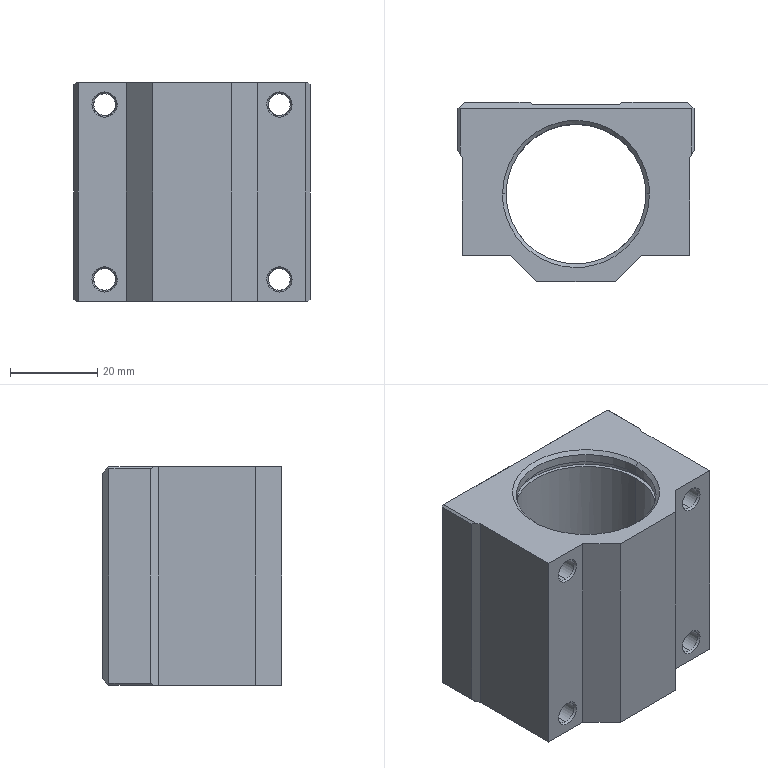Part | STEP file | _LHBB20-1_b | 1 solid | 80 faces | box 54 x 41 x 50 mm | volume 55289 mm3 | plane 34 | cylinder 26 | cone 20 | commonest cylinder face diameters 4.917 x8 5.2 x8 32 x6 33.7 x4